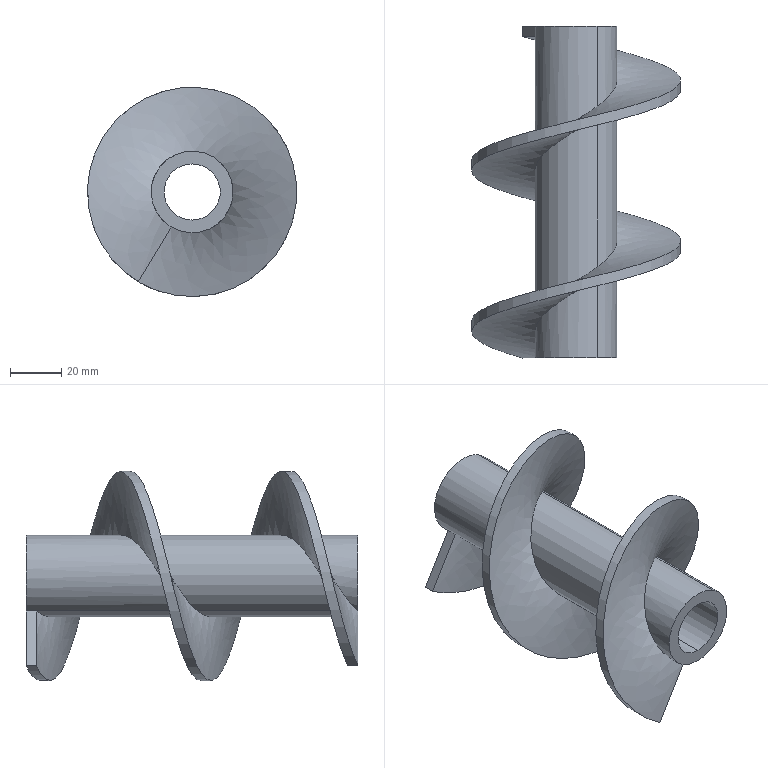Part | SolidWorks | features ICE 3, BaseBody 1, HoleWzd 1 | 1 solid | 15 faces | box 82 x 130 x 82 mm | volume 90947 mm3 | cylinder 8 | plane 4 | spline 3 | commonest cylinder face diameters 32 x6 22 x2